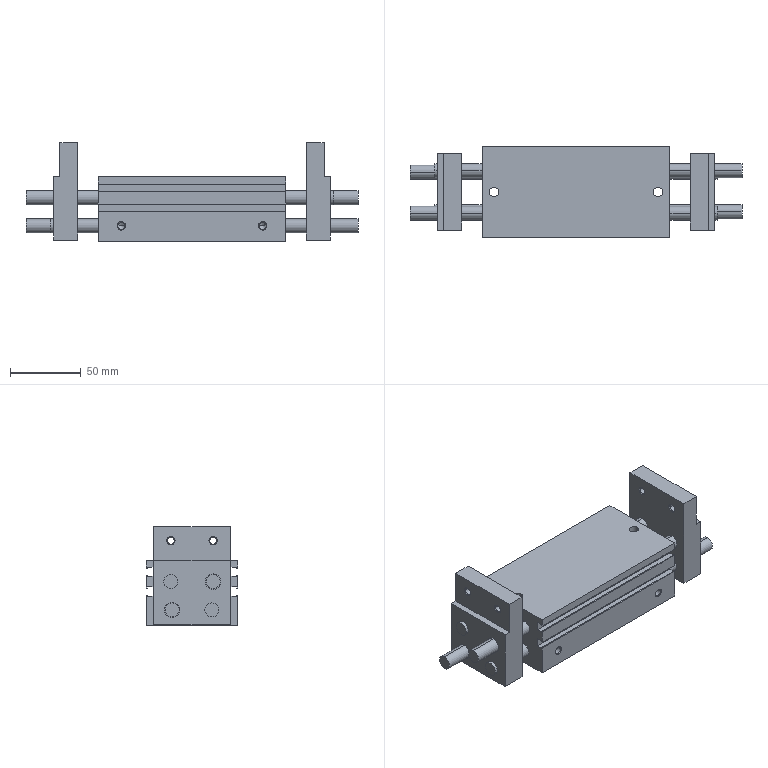Part | STEP file | ASND-0110-1-5 | 1 solid | 180 faces | box 235 x 65 x 70 mm | volume 504117 mm3 | plane 68 | cylinder 66 | cone 46 | commonest cylinder face diameters 10 x24 4.92 x20 11 x8 4 x4 4.13 x4 6.6 x4